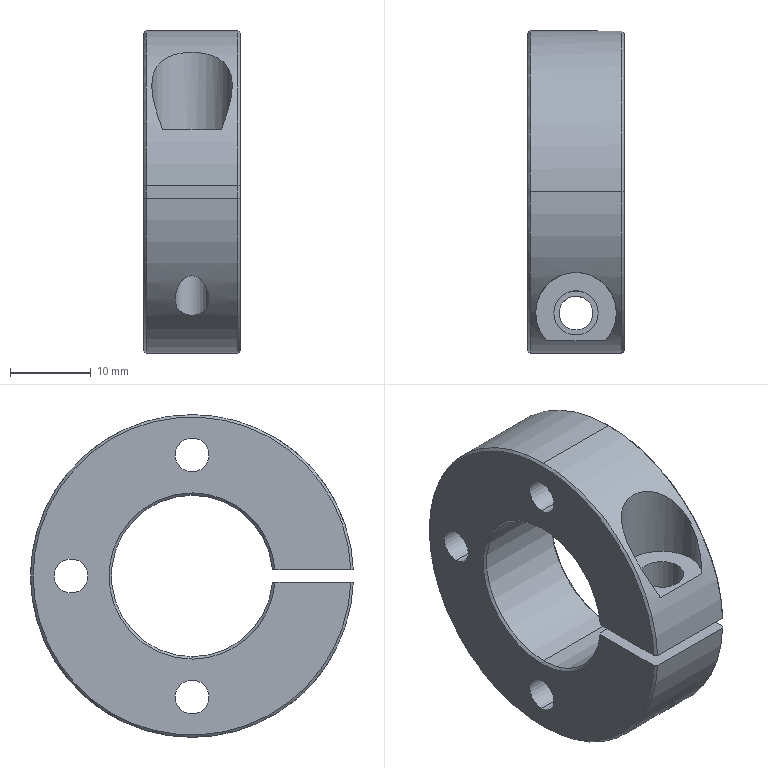Part | STEP file | SCSTR20-12_SCSTR20-12_1-2 | 1 solid | 35 faces | box 12 x 39.986 x 40 mm | volume 9883 mm3 | cylinder 19 | cone 11 | plane 5 | commonest cylinder face diameters 4.2 x8 10 x3 20 x3 40 x3 5.5 x2
STEP:
#1=CARTESIAN_POINT('',(-6.,0.,-17.1));
#2=VERTEX_POINT('',#1);
#3=CARTESIAN_POINT('',(-6.,0.,-12.9));
#4=VERTEX_POINT('',#3);
#5=CARTESIAN_POINT('',(-6.,0.,-15.));
#6=DIRECTION('',(-1.,0.,0.));
#7=DIRECTION('',(0.,0.,-1.));
#8=AXIS2_PLACEMENT_3D('',#5,#6,#7);
#9=CIRCLE('',#8,2.1);
#10=EDGE_CURVE('',#2,#4,#9,.T.);
#11=ORIENTED_EDGE('',*,*,#10,.T.);
#12=CARTESIAN_POINT('',(6.,0.,-12.9));
#13=VERTEX_POINT('',#12);
#14=CARTESIAN_POINT('',(6.,0.,-12.9));
#15=DIRECTION('',(1.,0.,0.));
#16=VECTOR('',#15,1000.);
#17=LINE('',#14,#16);
#18=EDGE_CURVE('',#4,#13,#17,.T.);
#19=ORIENTED_EDGE('',*,*,#18,.T.);
#20=CARTESIAN_POINT('',(6.,0.,-17.1));
#21=VERTEX_POINT('',#20);
#22=CARTESIAN_POINT('',(6.,0.,-15.));
#23=DIRECTION('',(-1.,0.,0.));
#24=DIRECTION('',(0.,0.,-1.));
#25=AXIS2_PLACEMENT_3D('',#22,#23,#24);
#26=CIRCLE('',#25,2.1);
#27=EDGE_CURVE('',#21,#13,#26,.T.);
#28=ORIENTED_EDGE('',*,*,#27,.F.);
#29=CARTESIAN_POINT('',(6.,0.,-17.1));
#30=DIRECTION('',(1.,0.,0.));
#31=VECTOR('',#30,1000.);
#32=LINE('',#29,#31);
#33=EDGE_CURVE('',#2,#21,#32,.T.);
#34=ORIENTED_EDGE('',*,*,#33,.F.);
#35=EDGE_LOOP('',(#11,#19,#28,#34));
#36=FACE_OUTER_BOUND('',#35,.T.);
#37=CARTESIAN_POINT('',(6.,0.,-15.));
#38=DIRECTION('',(1.,0.,0.));
#39=DIRECTION('',(0.,0.,-1.));
#40=AXIS2_PLACEMENT_3D('',#37,#38,#39);
#41=CYLINDRICAL_SURFACE('',#40,2.1);
#42=ADVANCED_FACE('',(#36),#41,.F.);
#43=CARTESIAN_POINT('',(-6.,0.,12.9));
#44=VERTEX_POINT('',#43);
#45=CARTESIAN_POINT('',(-6.,0.,17.1));
#46=VERTEX_POINT('',#45);
#47=CARTESIAN_POINT('',(-6.,0.,15.));
#48=DIRECTION('',(-1.,0.,0.));
#49=DIRECTION('',(0.,0.,-1.));
#50=AXIS2_PLACEMENT_3D('',#47,#48,#49);
#51=CIRCLE('',#50,2.1);
#52=EDGE_CURVE('',#44,#46,#51,.T.);
#53=ORIENTED_EDGE('',*,*,#52,.T.);
#54=CARTESIAN_POINT('',(6.,0.,17.1));
#55=VERTEX_POINT('',#54);
#56=CARTESIAN_POINT('',(6.,0.,17.1));
#57=DIRECTION('',(1.,0.,0.));
#58=VECTOR('',#57,1000.);
#59=LINE('',#56,#58);
#60=EDGE_CURVE('',#46,#55,#59,.T.);
#61=ORIENTED_EDGE('',*,*,#60,.T.);
#62=CARTESIAN_POINT('',(6.,0.,12.9));
#63=VERTEX_POINT('',#62);
#64=CARTESIAN_POINT('',(6.,0.,15.));
#65=DIRECTION('',(-1.,0.,0.));
#66=DIRECTION('',(0.,0.,-1.));
#67=AXIS2_PLACEMENT_3D('',#64,#65,#66);
#68=CIRCLE('',#67,2.1);
#69=EDGE_CURVE('',#63,#55,#68,.T.);
#70=ORIENTED_EDGE('',*,*,#69,.F.);
#71=CARTESIAN_POINT('',(6.,0.,12.9));
#72=DIRECTION('',(1.,0.,0.));
#73=VECTOR('',#72,1000.);
#74=LINE('',#71,#73);
#75=EDGE_CURVE('',#44,#63,#74,.T.);
#76=ORIENTED_EDGE('',*,*,#75,.F.);
#77=EDGE_LOOP('',(#53,#61,#70,#76));
#78=FACE_OUTER_BOUND('',#77,.T.);
#79=CARTESIAN_POINT('',(6.,0.,15.));
#80=DIRECTION('',(1.,0.,0.));
#81=DIRECTION('',(0.,0.,-1.));
#82=AXIS2_PLACEMENT_3D('',#79,#80,#81);
#83=CYLINDRICAL_SURFACE('',#82,2.1);
#84=ADVANCED_FACE('',(#78),#83,.F.);
#85=CARTESIAN_POINT('',(-6.,15.,-2.1));
#86=VERTEX_POINT('',#85);
#87=CARTESIAN_POINT('',(-6.,15.,2.1));
#88=VERTEX_POINT('',#87);
#89=CARTESIAN_POINT('',(-6.,15.,0.));
#90=DIRECTION('',(-1.,0.,0.));
#91=DIRECTION('',(0.,0.,-1.));
#92=AXIS2_PLACEMENT_3D('',#89,#90,#91);
#93=CIRCLE('',#92,2.1);
#94=EDGE_CURVE('',#86,#88,#93,.T.);
#95=ORIENTED_EDGE('',*,*,#94,.T.);
#96=CARTESIAN_POINT('',(6.,15.,2.1));
#97=VERTEX_POINT('',#96);
#98=CARTESIAN_POINT('',(6.,15.,2.1));
#99=DIRECTION('',(1.,0.,0.));
#100=VECTOR('',#99,1000.);
#101=LINE('',#98,#100);
#102=EDGE_CURVE('',#88,#97,#101,.T.);
#103=ORIENTED_EDGE('',*,*,#102,.T.);
#104=CARTESIAN_POINT('',(6.,15.,-2.1));
#105=VERTEX_POINT('',#104);
#106=CARTESIAN_POINT('',(6.,15.,0.));
#107=DIRECTION('',(-1.,0.,0.));
#108=DIRECTION('',(0.,0.,-1.));
#109=AXIS2_PLACEMENT_3D('',#106,#107,#108);
#110=CIRCLE('',#109,2.1);
#111=EDGE_CURVE('',#105,#97,#110,.T.);
#112=ORIENTED_EDGE('',*,*,#111,.F.);
#113=CARTESIAN_POINT('',(6.,15.,-2.1));
#114=DIRECTION('',(1.,0.,0.));
#115=VECTOR('',#114,1000.);
#116=LINE('',#113,#115);
#117=EDGE_CURVE('',#86,#105,#116,.T.);
#118=ORIENTED_EDGE('',*,*,#117,.F.);
#119=EDGE_LOOP('',(#95,#103,#112,#118));
#120=FACE_OUTER_BOUND('',#119,.T.);
#121=CARTESIAN_POINT('',(6.,15.,0.));
#122=DIRECTION('',(1.,0.,0.));
#123=DIRECTION('',(0.,0.,-1.));
#124=AXIS2_PLACEMENT_3D('',#121,#122,#123);
#125=CYLINDRICAL_SURFACE('',#124,2.1);
#126=ADVANCED_FACE('',(#120),#125,.F.);
#127=CARTESIAN_POINT('',(-5.7,0.,-10.));
#128=VERTEX_POINT('',#127);
#129=CARTESIAN_POINT('',(-5.7,-9.972,-0.75));
#130=VERTEX_POINT('',#129);
#131=CARTESIAN_POINT('',(-5.7,0.,0.));
#132=DIRECTION('',(-1.,0.,0.));
#133=DIRECTION('',(0.,0.,1.));
#134=AXIS2_PLACEMENT_3D('',#131,#132,#133);
#135=CIRCLE('',#134,10.);
#136=EDGE_CURVE('',#128,#130,#135,.T.);
#137=ORIENTED_EDGE('',*,*,#136,.F.);
#138=CARTESIAN_POINT('',(-6.,0.,-10.3));
#139=VERTEX_POINT('',#138);
#140=CARTESIAN_POINT('',(-6.,0.,-10.3));
#141=DIRECTION('',(-0.7071,0.,-0.7071));
#142=VECTOR('',#141,1000.);
#143=LINE('',#140,#142);
#144=EDGE_CURVE('',#128,#139,#143,.T.);
#145=ORIENTED_EDGE('',*,*,#144,.T.);
#146=CARTESIAN_POINT('',(-6.,-10.273,-0.75));
#147=VERTEX_POINT('',#146);
#148=CARTESIAN_POINT('',(-6.,0.,0.));
#149=DIRECTION('',(-1.,0.,0.));
#150=DIRECTION('',(0.,0.,1.));
#151=AXIS2_PLACEMENT_3D('',#148,#149,#150);
#152=CIRCLE('',#151,10.3);
#153=EDGE_CURVE('',#139,#147,#152,.T.);
#154=ORIENTED_EDGE('',*,*,#153,.T.);
#155=CARTESIAN_POINT('',(-6.,-10.273,-0.75));
#156=CARTESIAN_POINT('',(-5.9,-10.172,-0.75));
#157=CARTESIAN_POINT('',(-5.8,-10.072,-0.75));
#158=CARTESIAN_POINT('',(-5.7,-9.972,-0.75));
#159=B_SPLINE_CURVE_WITH_KNOTS('',3,(#155,#156,#157,#158),.UNSPECIFIED.,.F.,.F.,(4,4),(0.,0.0004248),.UNSPECIFIED.);
#160=EDGE_CURVE('',#147,#130,#159,.T.);
#161=ORIENTED_EDGE('',*,*,#160,.T.);
#162=EDGE_LOOP('',(#137,#145,#154,#161));
#163=FACE_OUTER_BOUND('',#162,.T.);
#164=CARTESIAN_POINT('',(-6.,0.,0.));
#165=DIRECTION('',(-1.,0.,0.));
#166=DIRECTION('',(0.,0.,1.));
#167=AXIS2_PLACEMENT_3D('',#164,#165,#166);
#168=CONICAL_SURFACE('',#167,10.3,0.7854);
#169=ADVANCED_FACE('',(#163),#168,.F.);
#170=ORIENTED_EDGE('',*,*,#144,.F.);
#171=CARTESIAN_POINT('',(-5.7,0.,10.));
#172=VERTEX_POINT('',#171);
#173=CARTESIAN_POINT('',(-5.7,0.,0.));
#174=DIRECTION('',(-1.,0.,0.));
#175=DIRECTION('',(0.,0.,1.));
#176=AXIS2_PLACEMENT_3D('',#173,#174,#175);
#177=CIRCLE('',#176,10.);
#178=EDGE_CURVE('',#172,#128,#177,.T.);
#179=ORIENTED_EDGE('',*,*,#178,.F.);
#180=CARTESIAN_POINT('',(-6.,0.,10.3));
#181=VERTEX_POINT('',#180);
#182=CARTESIAN_POINT('',(-6.,0.,10.3));
#183=DIRECTION('',(-0.7071,0.,0.7071));
#184=VECTOR('',#183,1000.);
#185=LINE('',#182,#184);
#186=EDGE_CURVE('',#172,#181,#185,.T.);
#187=ORIENTED_EDGE('',*,*,#186,.T.);
#188=CARTESIAN_POINT('',(-6.,0.,0.));
#189=DIRECTION('',(-1.,0.,0.));
#190=DIRECTION('',(0.,0.,1.));
#191=AXIS2_PLACEMENT_3D('',#188,#189,#190);
#192=CIRCLE('',#191,10.3);
#193=EDGE_CURVE('',#181,#139,#192,.T.);
#194=ORIENTED_EDGE('',*,*,#193,.T.);
#195=EDGE_LOOP('',(#170,#179,#187,#194));
#196=FACE_OUTER_BOUND('',#195,.T.);
#197=CARTESIAN_POINT('',(-6.,0.,0.));
#198=DIRECTION('',(-1.,0.,0.));
#199=DIRECTION('',(0.,0.,1.));
#200=AXIS2_PLACEMENT_3D('',#197,#198,#199);
#201=CONICAL_SURFACE('',#200,10.3,0.7854);
#202=ADVANCED_FACE('',(#196),#201,.F.);
#203=CARTESIAN_POINT('',(-6.,-19.686,-0.75));
#204=VERTEX_POINT('',#203);
#205=CARTESIAN_POINT('',(-6.,19.7,0.));
#206=VERTEX_POINT('',#205);
#207=CARTESIAN_POINT('',(-6.,0.,0.));
#208=DIRECTION('',(1.,0.,0.));
#209=DIRECTION('',(0.,0.,-1.));
#210=AXIS2_PLACEMENT_3D('',#207,#208,#209);
#211=CIRCLE('',#210,19.7);
#212=EDGE_CURVE('',#204,#206,#211,.T.);
#213=ORIENTED_EDGE('',*,*,#212,.T.);
#214=CARTESIAN_POINT('',(-5.7,20.,0.));
#215=VERTEX_POINT('',#214);
#216=CARTESIAN_POINT('',(-5.7,20.,0.));
#217=DIRECTION('',(0.7071,0.7071,0.));
#218=VECTOR('',#217,1000.);
#219=LINE('',#216,#218);
#220=EDGE_CURVE('',#206,#215,#219,.T.);
#221=ORIENTED_EDGE('',*,*,#220,.T.);
#222=CARTESIAN_POINT('',(-5.7,0.,-20.));
#223=VERTEX_POINT('',#222);
#224=CARTESIAN_POINT('',(-5.7,0.,0.));
#225=DIRECTION('',(-1.,0.,0.));
#226=DIRECTION('',(0.,0.,-1.));
#227=AXIS2_PLACEMENT_3D('',#224,#225,#226);
#228=CIRCLE('',#227,20.);
#229=EDGE_CURVE('',#215,#223,#228,.T.);
#230=ORIENTED_EDGE('',*,*,#229,.T.);
#231=CARTESIAN_POINT('',(-5.7,-19.986,-0.75));
#232=VERTEX_POINT('',#231);
#233=CARTESIAN_POINT('',(-5.7,0.,0.));
#234=DIRECTION('',(-1.,0.,0.));
#235=DIRECTION('',(0.,0.,-1.));
#236=AXIS2_PLACEMENT_3D('',#233,#234,#235);
#237=CIRCLE('',#236,20.);
#238=EDGE_CURVE('',#223,#232,#237,.T.);
#239=ORIENTED_EDGE('',*,*,#238,.T.);
#240=CARTESIAN_POINT('',(-5.7,-19.986,-0.75));
#241=CARTESIAN_POINT('',(-5.8,-19.886,-0.75));
#242=CARTESIAN_POINT('',(-5.9,-19.786,-0.75));
#243=CARTESIAN_POINT('',(-6.,-19.686,-0.75));
#244=B_SPLINE_CURVE_WITH_KNOTS('',3,(#240,#241,#242,#243),.UNSPECIFIED.,.F.,.F.,(4,4),(0.,0.0004244),.UNSPECIFIED.);
#245=EDGE_CURVE('',#232,#204,#244,.T.);
#246=ORIENTED_EDGE('',*,*,#245,.T.);
#247=EDGE_LOOP('',(#213,#221,#230,#239,#246));
#248=FACE_OUTER_BOUND('',#247,.T.);
#249=CARTESIAN_POINT('',(-5.7,0.,0.));
#250=DIRECTION('',(1.,0.,0.));
#251=DIRECTION('',(0.,1.,0.));
#252=AXIS2_PLACEMENT_3D('',#249,#250,#251);
#253=CONICAL_SURFACE('',#252,20.,0.7854);
#254=ADVANCED_FACE('',(#248),#253,.T.);
#255=CARTESIAN_POINT('',(-5.7,-9.972,0.75));
#256=VERTEX_POINT('',#255);
#257=CARTESIAN_POINT('',(-5.7,0.,0.));
#258=DIRECTION('',(-1.,0.,0.));
#259=DIRECTION('',(0.,0.,1.));
#260=AXIS2_PLACEMENT_3D('',#257,#258,#259);
#261=CIRCLE('',#260,10.);
#262=EDGE_CURVE('',#256,#172,#261,.T.);
#263=ORIENTED_EDGE('',*,*,#262,.T.);
#264=CARTESIAN_POINT('',(5.7,0.,10.));
#265=VERTEX_POINT('',#264);
#266=CARTESIAN_POINT('',(-6.,0.,10.));
#267=DIRECTION('',(1.,0.,0.));
#268=VECTOR('',#267,1000.);
#269=LINE('',#266,#268);
#270=EDGE_CURVE('',#172,#265,#269,.T.);
#271=ORIENTED_EDGE('',*,*,#270,.T.);
#272=CARTESIAN_POINT('',(5.7,-9.972,0.75));
#273=VERTEX_POINT('',#272);
#274=CARTESIAN_POINT('',(5.7,0.,0.));
#275=DIRECTION('',(-1.,0.,0.));
#276=DIRECTION('',(0.,0.,-1.));
#277=AXIS2_PLACEMENT_3D('',#274,#275,#276);
#278=CIRCLE('',#277,10.);
#279=EDGE_CURVE('',#273,#265,#278,.T.);
#280=ORIENTED_EDGE('',*,*,#279,.F.);
#281=CARTESIAN_POINT('',(-6.,-9.972,0.75));
#282=DIRECTION('',(-1.,0.,0.));
#283=VECTOR('',#282,1000.);
#284=LINE('',#281,#283);
#285=EDGE_CURVE('',#273,#256,#284,.T.);
#286=ORIENTED_EDGE('',*,*,#285,.T.);
#287=EDGE_LOOP('',(#263,#271,#280,#286));
#288=FACE_OUTER_BOUND('',#287,.T.);
#289=CARTESIAN_POINT('',(-6.,0.,0.));
#290=DIRECTION('',(1.,0.,0.));
#291=DIRECTION('',(0.,0.,-1.));
#292=AXIS2_PLACEMENT_3D('',#289,#290,#291);
#293=CYLINDRICAL_SURFACE('',#292,10.);
#294=ADVANCED_FACE('',(#288),#293,.F.);
#295=ORIENTED_EDGE('',*,*,#270,.F.);
#296=ORIENTED_EDGE('',*,*,#178,.T.);
#297=CARTESIAN_POINT('',(5.7,0.,-10.));
#298=VERTEX_POINT('',#297);
#299=CARTESIAN_POINT('',(-6.,0.,-10.));
#300=DIRECTION('',(1.,0.,0.));
#301=VECTOR('',#300,1000.);
#302=LINE('',#299,#301);
#303=EDGE_CURVE('',#128,#298,#302,.T.);
#304=ORIENTED_EDGE('',*,*,#303,.T.);
#305=CARTESIAN_POINT('',(5.7,0.,0.));
#306=DIRECTION('',(-1.,0.,0.));
#307=DIRECTION('',(0.,0.,-1.));
#308=AXIS2_PLACEMENT_3D('',#305,#306,#307);
#309=CIRCLE('',#308,10.);
#310=EDGE_CURVE('',#265,#298,#309,.T.);
#311=ORIENTED_EDGE('',*,*,#310,.F.);
#312=EDGE_LOOP('',(#295,#296,#304,#311));
#313=FACE_OUTER_BOUND('',#312,.T.);
#314=CARTESIAN_POINT('',(-6.,0.,0.));
#315=DIRECTION('',(1.,0.,0.));
#316=DIRECTION('',(0.,0.,-1.));
#317=AXIS2_PLACEMENT_3D('',#314,#315,#316);
#318=CYLINDRICAL_SURFACE('',#317,10.);
#319=ADVANCED_FACE('',(#313),#318,.F.);
#320=CARTESIAN_POINT('',(2.75,-15.,7.75));
#321=VERTEX_POINT('',#320);
#322=CARTESIAN_POINT('',(-2.75,-15.,7.75));
#323=VERTEX_POINT('',#322);
#324=CARTESIAN_POINT('',(0.,-15.,7.75));
#325=DIRECTION('',(0.,0.,-1.));
#326=DIRECTION('',(-1.,0.,0.));
#327=AXIS2_PLACEMENT_3D('',#324,#325,#326);
#328=CIRCLE('',#327,2.75);
#329=EDGE_CURVE('',#321,#323,#328,.T.);
#330=ORIENTED_EDGE('',*,*,#329,.F.);
#331=CARTESIAN_POINT('',(2.75,-15.,0.75));
#332=VERTEX_POINT('',#331);
#333=CARTESIAN_POINT('',(2.75,-15.,0.75));
#334=DIRECTION('',(0.,0.,-1.));
#335=VECTOR('',#334,1000.);
#336=LINE('',#333,#335);
#337=EDGE_CURVE('',#321,#332,#336,.T.);
#338=ORIENTED_EDGE('',*,*,#337,.T.);
#339=CARTESIAN_POINT('',(-2.75,-15.,0.75));
#340=VERTEX_POINT('',#339);
#341=CARTESIAN_POINT('',(0.,-15.,0.75));
#342=DIRECTION('',(0.,0.,-1.));
#343=DIRECTION('',(-1.,0.,0.));
#344=AXIS2_PLACEMENT_3D('',#341,#342,#343);
#345=CIRCLE('',#344,2.75);
#346=EDGE_CURVE('',#332,#340,#345,.T.);
#347=ORIENTED_EDGE('',*,*,#346,.T.);
#348=CARTESIAN_POINT('',(-2.75,-15.,0.75));
#349=DIRECTION('',(0.,0.,-1.));
#350=VECTOR('',#349,1000.);
#351=LINE('',#348,#350);
#352=EDGE_CURVE('',#323,#340,#351,.T.);
#353=ORIENTED_EDGE('',*,*,#352,.F.);
#354=EDGE_LOOP('',(#330,#338,#347,#353));
#355=FACE_OUTER_BOUND('',#354,.T.);
#356=CARTESIAN_POINT('',(0.,-15.,0.75));
#357=DIRECTION('',(0.,0.,-1.));
#358=DIRECTION('',(-1.,0.,0.));
#359=AXIS2_PLACEMENT_3D('',#356,#357,#358);
#360=CYLINDRICAL_SURFACE('',#359,2.75);
#361=ADVANCED_FACE('',(#355),#360,.F.);
#362=CARTESIAN_POINT('',(5.7,0.,20.));
#363=VERTEX_POINT('',#362);
#364=CARTESIAN_POINT('',(5.7,0.,-20.));
#365=VERTEX_POINT('',#364);
#366=CARTESIAN_POINT('',(5.7,0.,0.));
#367=DIRECTION('',(-1.,0.,0.));
#368=DIRECTION('',(0.,0.,1.));
#369=AXIS2_PLACEMENT_3D('',#366,#367,#368);
#370=CIRCLE('',#369,20.);
#371=EDGE_CURVE('',#363,#365,#370,.T.);
#372=ORIENTED_EDGE('',*,*,#371,.T.);
#373=CARTESIAN_POINT('',(6.,0.,-20.));
#374=DIRECTION('',(-1.,0.,0.));
#375=VECTOR('',#374,1000.);
#376=LINE('',#373,#375);
#377=EDGE_CURVE('',#365,#223,#376,.T.);
#378=ORIENTED_EDGE('',*,*,#377,.T.);
#379=ORIENTED_EDGE('',*,*,#229,.F.);
#380=CARTESIAN_POINT('',(-5.7,0.,20.));
#381=VERTEX_POINT('',#380);
#382=CARTESIAN_POINT('',(-5.7,0.,0.));
#383=DIRECTION('',(-1.,0.,0.));
#384=DIRECTION('',(0.,0.,-1.));
#385=AXIS2_PLACEMENT_3D('',#382,#383,#384);
#386=CIRCLE('',#385,20.);
#387=EDGE_CURVE('',#381,#215,#386,.T.);
#388=ORIENTED_EDGE('',*,*,#387,.F.);
#389=CARTESIAN_POINT('',(6.,0.,20.));
#390=DIRECTION('',(-1.,0.,0.));
#391=VECTOR('',#390,1000.);
#392=LINE('',#389,#391);
#393=EDGE_CURVE('',#363,#381,#392,.T.);
#394=ORIENTED_EDGE('',*,*,#393,.F.);
#395=EDGE_LOOP('',(#372,#378,#379,#388,#394));
#396=FACE_OUTER_BOUND('',#395,.T.);
#397=CARTESIAN_POINT('',(6.,0.,0.));
#398=DIRECTION('',(-1.,0.,0.));
#399=DIRECTION('',(0.,0.,1.));
#400=AXIS2_PLACEMENT_3D('',#397,#398,#399);
#401=CYLINDRICAL_SURFACE('',#400,20.);
#402=ADVANCED_FACE('',(#396),#401,.T.);
#403=CARTESIAN_POINT('',(-3.631,-18.437,7.75));
#404=VERTEX_POINT('',#403);
#405=CARTESIAN_POINT('',(-5.,-15.,13.229));
#406=VERTEX_POINT('',#405);
#407=CARTESIAN_POINT('',(-3.631,-18.437,7.75));
#408=CARTESIAN_POINT('',(-4.016,-18.03,8.718));
#409=CARTESIAN_POINT('',(-4.348,-17.547,9.658));
#410=CARTESIAN_POINT('',(-4.716,-16.691,11.033));
#411=CARTESIAN_POINT('',(-4.817,-16.383,11.485));
#412=CARTESIAN_POINT('',(-4.96,-15.719,12.378));
#413=CARTESIAN_POINT('',(-5.,-15.368,12.811));
#414=CARTESIAN_POINT('',(-5.,-15.,13.229));
#415=B_SPLINE_CURVE_WITH_KNOTS('',3,(#407,#408,#409,#410,#411,#412,#413,#414),.UNSPECIFIED.,.F.,.F.,(4,2,2,4),(-0.01582,-0.01247,-0.0108,-0.009124),.UNSPECIFIED.);
#416=EDGE_CURVE('',#404,#406,#415,.T.);
#417=ORIENTED_EDGE('',*,*,#416,.T.);
#418=CARTESIAN_POINT('',(5.,-15.,13.229));
#419=VERTEX_POINT('',#418);
#420=CARTESIAN_POINT('',(-5.,-15.,13.229));
#421=CARTESIAN_POINT('',(-5.,-14.75,13.513));
#422=CARTESIAN_POINT('',(-4.981,-14.491,13.79));
#423=CARTESIAN_POINT('',(-4.897,-13.957,14.33));
#424=CARTESIAN_POINT('',(-4.832,-13.684,14.59));
#425=CARTESIAN_POINT('',(-4.65,-13.139,15.083));
#426=CARTESIAN_POINT('',(-4.532,-12.865,15.317));
#427=CARTESIAN_POINT('',(-4.232,-12.319,15.76));
#428=CARTESIAN_POINT('',(-4.051,-12.05,15.965));
#429=CARTESIAN_POINT('',(-3.733,-11.669,16.243));
#430=CARTESIAN_POINT('',(-3.619,-11.546,16.332));
#431=CARTESIAN_POINT('',(-3.374,-11.306,16.499));
#432=CARTESIAN_POINT('',(-3.241,-11.189,16.578));
#433=CARTESIAN_POINT('',(-2.827,-10.861,16.796));
#434=CARTESIAN_POINT('',(-2.525,-10.669,16.918));
#435=CARTESIAN_POINT('',(-2.031,-10.427,17.067));
#436=CARTESIAN_POINT('',(-1.858,-10.354,17.111));
#437=CARTESIAN_POINT('',(-1.504,-10.228,17.187));
#438=CARTESIAN_POINT('',(-1.324,-10.175,17.218));
#439=CARTESIAN_POINT('',(-0.9586,-10.089,17.269));
#440=CARTESIAN_POINT('',(-0.7727,-10.056,17.288));
#441=CARTESIAN_POINT('',(-0.3947,-10.012,17.314));
#442=CARTESIAN_POINT('',(-0.2017,-10.,17.32));
#443=CARTESIAN_POINT('',(0.3765,-9.999,17.321));
#444=CARTESIAN_POINT('',(0.7534,-10.043,17.296));
#445=CARTESIAN_POINT('',(1.306,-10.17,17.221));
#446=CARTESIAN_POINT('',(1.489,-10.223,17.19));
#447=CARTESIAN_POINT('',(1.843,-10.348,17.115));
#448=CARTESIAN_POINT('',(2.014,-10.42,17.071));
#449=CARTESIAN_POINT('',(2.51,-10.66,16.923));
#450=CARTESIAN_POINT('',(2.821,-10.857,16.799));
#451=CARTESIAN_POINT('',(3.374,-11.293,16.508));
#452=CARTESIAN_POINT('',(3.619,-11.534,16.342));
#453=CARTESIAN_POINT('',(4.05,-12.049,15.967));
#454=CARTESIAN_POINT('',(4.229,-12.315,15.763));
#455=CARTESIAN_POINT('',(4.53,-12.86,15.321));
#456=CARTESIAN_POINT('',(4.65,-13.139,15.083));
#457=CARTESIAN_POINT('',(4.833,-13.686,14.588));
#458=CARTESIAN_POINT('',(4.897,-13.956,14.331));
#459=CARTESIAN_POINT('',(4.981,-14.486,13.795));
#460=CARTESIAN_POINT('',(5.,-14.748,13.515));
#461=CARTESIAN_POINT('',(5.,-15.,13.229));
#462=B_SPLINE_CURVE_WITH_KNOTS('',3,(#420,#421,#422,#423,#424,#425,#426,#427,#428,#429,#430,#431,#432,#433,#434,#435,#436,#437,#438,#439,#440,#441,#442,#443,#444,#445,#446,#447,#448,#449,#450,#451,#452,#453,#454,#455,#456,#457,#458,#459,#460,#461),.UNSPECIFIED.,.F.,.F.,(4,2,2,2,2,2,2,2,2,2,2,2,2,2,2,2,2,2,2,2,4),(-0.009124,-0.007984,-0.006845,-0.005706,-0.004566,-0.003997,-0.003427,-0.002288,-0.001718,-0.001148,-0.0005785,-0.00000887,0.00113,0.0017,0.00227,0.003409,0.004549,0.005688,0.006827,0.007967,0.009106),.UNSPECIFIED.);
#463=EDGE_CURVE('',#406,#419,#462,.T.);
#464=ORIENTED_EDGE('',*,*,#463,.T.);
#465=CARTESIAN_POINT('',(3.631,-18.437,7.75));
#466=VERTEX_POINT('',#465);
#467=CARTESIAN_POINT('',(5.,-15.,13.229));
#468=CARTESIAN_POINT('',(5.,-15.369,12.81));
#469=CARTESIAN_POINT('',(4.96,-15.717,12.381));
#470=CARTESIAN_POINT('',(4.82,-16.372,11.5));
#471=CARTESIAN_POINT('',(4.72,-16.68,11.049));
#472=CARTESIAN_POINT('',(4.473,-17.256,10.125));
#473=CARTESIAN_POINT('',(4.327,-17.522,9.657));
#474=CARTESIAN_POINT('',(4.003,-18.011,8.711));
#475=CARTESIAN_POINT('',(3.823,-18.234,8.234));
#476=CARTESIAN_POINT('',(3.631,-18.437,7.75));
#477=B_SPLINE_CURVE_WITH_KNOTS('',3,(#467,#468,#469,#470,#471,#472,#473,#474,#475,#476),.UNSPECIFIED.,.F.,.F.,(4,2,2,2,4),(0.009106,0.01078,0.01244,0.01411,0.01578),.UNSPECIFIED.);
#478=EDGE_CURVE('',#419,#466,#477,.T.);
#479=ORIENTED_EDGE('',*,*,#478,.T.);
#480=CARTESIAN_POINT('',(6.,-18.437,7.75));
#481=DIRECTION('',(-1.,0.,0.));
#482=VECTOR('',#481,1000.);
#483=LINE('',#480,#482);
#484=EDGE_CURVE('',#466,#404,#483,.T.);
#485=ORIENTED_EDGE('',*,*,#484,.T.);
#486=EDGE_LOOP('',(#417,#464,#479,#485));
#487=FACE_BOUND('',#486,.T.);
#488=CARTESIAN_POINT('',(5.7,-19.986,0.75));
#489=VERTEX_POINT('',#488);
#490=CARTESIAN_POINT('',(5.7,0.,0.));
#491=DIRECTION('',(-1.,0.,0.));
#492=DIRECTION('',(0.,0.,1.));
#493=AXIS2_PLACEMENT_3D('',#490,#491,#492);
#494=CIRCLE('',#493,20.);
#495=EDGE_CURVE('',#489,#363,#494,.T.);
#496=ORIENTED_EDGE('',*,*,#495,.T.);
#497=ORIENTED_EDGE('',*,*,#393,.T.);
#498=CARTESIAN_POINT('',(-5.7,-19.986,0.75));
#499=VERTEX_POINT('',#498);
#500=CARTESIAN_POINT('',(-5.7,0.,0.));
#501=DIRECTION('',(-1.,0.,0.));
#502=DIRECTION('',(0.,0.,-1.));
#503=AXIS2_PLACEMENT_3D('',#500,#501,#502);
#504=CIRCLE('',#503,20.);
#505=EDGE_CURVE('',#499,#381,#504,.T.);
#506=ORIENTED_EDGE('',*,*,#505,.F.);
#507=CARTESIAN_POINT('',(-6.,-19.986,0.75));
#508=DIRECTION('',(1.,0.,0.));
#509=VECTOR('',#508,1000.);
#510=LINE('',#507,#509);
#511=EDGE_CURVE('',#499,#489,#510,.T.);
#512=ORIENTED_EDGE('',*,*,#511,.T.);
#513=EDGE_LOOP('',(#496,#497,#506,#512));
#514=FACE_OUTER_BOUND('',#513,.T.);
#515=CARTESIAN_POINT('',(6.,0.,0.));
#516=DIRECTION('',(-1.,0.,0.));
#517=DIRECTION('',(0.,0.,1.));
#518=AXIS2_PLACEMENT_3D('',#515,#516,#517);
#519=CYLINDRICAL_SURFACE('',#518,20.);
#520=ADVANCED_FACE('',(#487,#514),#519,.T.);
#521=CARTESIAN_POINT('',(-2.1,-15.,-13.229));
#522=VERTEX_POINT('',#521);
#523=CARTESIAN_POINT('',(2.1,-15.,-13.229));
#524=VERTEX_POINT('',#523);
#525=CARTESIAN_POINT('',(-2.1,-15.,-13.229));
#526=CARTESIAN_POINT('',(-2.1,-15.248,-12.947));
#527=CARTESIAN_POINT('',(-2.057,-15.484,-12.664));
#528=CARTESIAN_POINT('',(-1.897,-15.932,-12.096));
#529=CARTESIAN_POINT('',(-1.777,-16.146,-11.807));
#530=CARTESIAN_POINT('',(-1.537,-16.436,-11.396));
#531=CARTESIAN_POINT('',(-1.447,-16.528,-11.262));
#532=CARTESIAN_POINT('',(-1.238,-16.702,-11.003));
#533=CARTESIAN_POINT('',(-1.121,-16.782,-10.88));
#534=CARTESIAN_POINT('',(-0.8546,-16.924,-10.658));
#535=CARTESIAN_POINT('',(-0.7046,-16.986,-10.559));
#536=CARTESIAN_POINT('',(-0.37,-17.074,-10.415));
#537=CARTESIAN_POINT('',(-0.183,-17.1,-10.372));
#538=CARTESIAN_POINT('',(0.1932,-17.1,-10.373));
#539=CARTESIAN_POINT('',(0.379,-17.073,-10.418));
#540=CARTESIAN_POINT('',(0.7112,-16.983,-10.563));
#541=CARTESIAN_POINT('',(0.8616,-16.921,-10.663));
#542=CARTESIAN_POINT('',(1.125,-16.779,-10.884));
#543=CARTESIAN_POINT('',(1.243,-16.698,-11.009));
#544=CARTESIAN_POINT('',(1.45,-16.525,-11.267));
#545=CARTESIAN_POINT('',(1.54,-16.434,-11.4));
#546=CARTESIAN_POINT('',(1.779,-16.144,-11.811));
#547=CARTESIAN_POINT('',(1.898,-15.93,-12.098));
#548=CARTESIAN_POINT('',(2.057,-15.483,-12.665));
#549=CARTESIAN_POINT('',(2.1,-15.248,-12.948));
#550=CARTESIAN_POINT('',(2.1,-15.,-13.229));
#551=B_SPLINE_CURVE_WITH_KNOTS('',3,(#525,#526,#527,#528,#529,#530,#531,#532,#533,#534,#535,#536,#537,#538,#539,#540,#541,#542,#543,#544,#545,#546,#547,#548,#549,#550),.UNSPECIFIED.,.F.,.F.,(4,2,2,2,2,2,2,2,2,2,2,2,4),(0.007926,0.009035,0.01014,0.0107,0.01125,0.01181,0.01236,0.01292,0.01347,0.01402,0.01458,0.01569,0.0168),.UNSPECIFIED.);
#552=EDGE_CURVE('',#522,#524,#551,.T.);
#553=ORIENTED_EDGE('',*,*,#552,.F.);
#554=CARTESIAN_POINT('',(-2.1,-15.,-0.75));
#555=VERTEX_POINT('',#554);
#556=CARTESIAN_POINT('',(-2.1,-15.,-0.75));
#557=DIRECTION('',(0.,0.,1.));
#558=VECTOR('',#557,1000.);
#559=LINE('',#556,#558);
#560=EDGE_CURVE('',#522,#555,#559,.T.);
#561=ORIENTED_EDGE('',*,*,#560,.T.);
#562=CARTESIAN_POINT('',(2.1,-15.,-0.75));
#563=VERTEX_POINT('',#562);
#564=CARTESIAN_POINT('',(0.,-15.,-0.75));
#565=DIRECTION('',(0.,0.,1.));
#566=DIRECTION('',(1.,0.,0.));
#567=AXIS2_PLACEMENT_3D('',#564,#565,#566);
#568=CIRCLE('',#567,2.1);
#569=EDGE_CURVE('',#555,#563,#568,.T.);
#570=ORIENTED_EDGE('',*,*,#569,.T.);
#571=CARTESIAN_POINT('',(2.1,-15.,-0.75));
#572=DIRECTION('',(0.,0.,1.));
#573=VECTOR('',#572,1000.);
#574=LINE('',#571,#573);
#575=EDGE_CURVE('',#524,#563,#574,.T.);
#576=ORIENTED_EDGE('',*,*,#575,.F.);
#577=EDGE_LOOP('',(#553,#561,#570,#576));
#578=FACE_OUTER_BOUND('',#577,.T.);
#579=CARTESIAN_POINT('',(0.,-15.,-0.75));
#580=DIRECTION('',(0.,0.,1.));
#581=DIRECTION('',(1.,0.,0.));
#582=AXIS2_PLACEMENT_3D('',#579,#580,#581);
#583=CYLINDRICAL_SURFACE('',#582,2.1);
#584=ADVANCED_FACE('',(#578),#583,.F.);
#585=CARTESIAN_POINT('',(6.,0.,-19.7));
#586=VERTEX_POINT('',#585);
#587=CARTESIAN_POINT('',(6.,0.,19.7));
#588=VERTEX_POINT('',#587);
#589=CARTESIAN_POINT('',(6.,0.,0.));
#590=DIRECTION('',(1.,0.,0.));
#591=DIRECTION('',(0.,0.,1.));
#592=AXIS2_PLACEMENT_3D('',#589,#590,#591);
#593=CIRCLE('',#592,19.7);
#594=EDGE_CURVE('',#586,#588,#593,.T.);
#595=ORIENTED_EDGE('',*,*,#594,.F.);
#596=CARTESIAN_POINT('',(5.7,0.,-20.));
#597=DIRECTION('',(-0.7071,0.,-0.7071));
#598=VECTOR('',#597,1000.);
#599=LINE('',#596,#598);
#600=EDGE_CURVE('',#586,#365,#599,.T.);
#601=ORIENTED_EDGE('',*,*,#600,.T.);
#602=ORIENTED_EDGE('',*,*,#371,.F.);
#603=CARTESIAN_POINT('',(5.7,0.,20.));
#604=DIRECTION('',(-0.7071,0.,0.7071));
#605=VECTOR('',#604,1000.);
#606=LINE('',#603,#605);
#607=EDGE_CURVE('',#588,#363,#606,.T.);
#608=ORIENTED_EDGE('',*,*,#607,.F.);
#609=EDGE_LOOP('',(#595,#601,#602,#608));
#610=FACE_OUTER_BOUND('',#609,.T.);
#611=CARTESIAN_POINT('',(5.7,0.,0.));
#612=DIRECTION('',(-1.,0.,0.));
#613=DIRECTION('',(0.,0.,1.));
#614=AXIS2_PLACEMENT_3D('',#611,#612,#613);
#615=CONICAL_SURFACE('',#614,20.,0.7854);
#616=ADVANCED_FACE('',(#610),#615,.T.);
#617=CARTESIAN_POINT('',(6.,-19.686,0.75));
#618=VERTEX_POINT('',#617);
#619=CARTESIAN_POINT('',(6.,0.,0.));
#620=DIRECTION('',(1.,0.,0.));
#621=DIRECTION('',(0.,0.,1.));
#622=AXIS2_PLACEMENT_3D('',#619,#620,#621);
#623=CIRCLE('',#622,19.7);
#624=EDGE_CURVE('',#588,#618,#623,.T.);
#625=ORIENTED_EDGE('',*,*,#624,.F.);
#626=ORIENTED_EDGE('',*,*,#607,.T.);
#627=ORIENTED_EDGE('',*,*,#495,.F.);
#628=CARTESIAN_POINT('',(5.7,-19.986,0.75));
#629=CARTESIAN_POINT('',(5.8,-19.886,0.75));
#630=CARTESIAN_POINT('',(5.9,-19.786,0.75));
#631=CARTESIAN_POINT('',(6.,-19.686,0.75));
#632=B_SPLINE_CURVE_WITH_KNOTS('',3,(#628,#629,#630,#631),.UNSPECIFIED.,.F.,.F.,(4,4),(0.,0.0004244),.UNSPECIFIED.);
#633=EDGE_CURVE('',#489,#618,#632,.T.);
#634=ORIENTED_EDGE('',*,*,#633,.T.);
#635=EDGE_LOOP('',(#625,#626,#627,#634));
#636=FACE_OUTER_BOUND('',#635,.T.);
#637=CARTESIAN_POINT('',(5.7,0.,0.));
#638=DIRECTION('',(-1.,0.,0.));
#639=DIRECTION('',(0.,0.,1.));
#640=AXIS2_PLACEMENT_3D('',#637,#638,#639);
#641=CONICAL_SURFACE('',#640,20.,0.7854);
#642=ADVANCED_FACE('',(#636),#641,.T.);
#643=ORIENTED_EDGE('',*,*,#279,.T.);
#644=CARTESIAN_POINT('',(6.,0.,10.3));
#645=VERTEX_POINT('',#644);
#646=CARTESIAN_POINT('',(6.,0.,10.3));
#647=DIRECTION('',(0.7071,0.,0.7071));
#648=VECTOR('',#647,1000.);
#649=LINE('',#646,#648);
#650=EDGE_CURVE('',#265,#645,#649,.T.);
#651=ORIENTED_EDGE('',*,*,#650,.T.);
#652=CARTESIAN_POINT('',(6.,-10.273,0.75));
#653=VERTEX_POINT('',#652);
#654=CARTESIAN_POINT('',(6.,0.,0.));
#655=DIRECTION('',(-1.,0.,0.));
#656=DIRECTION('',(0.,0.,-1.));
#657=AXIS2_PLACEMENT_3D('',#654,#655,#656);
#658=CIRCLE('',#657,10.3);
#659=EDGE_CURVE('',#653,#645,#658,.T.);
#660=ORIENTED_EDGE('',*,*,#659,.F.);
#661=CARTESIAN_POINT('',(5.7,-9.972,0.75));
#662=CARTESIAN_POINT('',(5.8,-10.072,0.75));
#663=CARTESIAN_POINT('',(5.9,-10.172,0.75));
#664=CARTESIAN_POINT('',(6.,-10.273,0.75));
#665=B_SPLINE_CURVE_WITH_KNOTS('',3,(#661,#662,#663,#664),.UNSPECIFIED.,.F.,.F.,(4,4),(0.,0.0004248),.UNSPECIFIED.);
#666=EDGE_CURVE('',#273,#653,#665,.T.);
#667=ORIENTED_EDGE('',*,*,#666,.F.);
#668=EDGE_LOOP('',(#643,#651,#660,#667));
#669=FACE_OUTER_BOUND('',#668,.T.);
#670=CARTESIAN_POINT('',(6.,0.,0.));
#671=DIRECTION('',(1.,0.,0.));
#672=DIRECTION('',(0.,0.,-1.));
#673=AXIS2_PLACEMENT_3D('',#670,#671,#672);
#674=CONICAL_SURFACE('',#673,10.3,0.7854);
#675=ADVANCED_FACE('',(#669),#674,.F.);
#676=ORIENTED_EDGE('',*,*,#650,.F.);
#677=ORIENTED_EDGE('',*,*,#310,.T.);
#678=CARTESIAN_POINT('',(6.,0.,-10.3));
#679=VERTEX_POINT('',#678);
#680=CARTESIAN_POINT('',(6.,0.,-10.3));
#681=DIRECTION('',(0.7071,0.,-0.7071));
#682=VECTOR('',#681,1000.);
#683=LINE('',#680,#682);
#684=EDGE_CURVE('',#298,#679,#683,.T.);
#685=ORIENTED_EDGE('',*,*,#684,.T.);
#686=CARTESIAN_POINT('',(6.,0.,0.));
#687=DIRECTION('',(-1.,0.,0.));
#688=DIRECTION('',(0.,0.,-1.));
#689=AXIS2_PLACEMENT_3D('',#686,#687,#688);
#690=CIRCLE('',#689,10.3);
#691=EDGE_CURVE('',#645,#679,#690,.T.);
#692=ORIENTED_EDGE('',*,*,#691,.F.);
#693=EDGE_LOOP('',(#676,#677,#685,#692));
#694=FACE_OUTER_BOUND('',#693,.T.);
#695=CARTESIAN_POINT('',(6.,0.,0.));
#696=DIRECTION('',(1.,0.,0.));
#697=DIRECTION('',(0.,0.,-1.));
#698=AXIS2_PLACEMENT_3D('',#695,#696,#697);
#699=CONICAL_SURFACE('',#698,10.3,0.7854);
#700=ADVANCED_FACE('',(#694),#699,.F.);
#701=ORIENTED_EDGE('',*,*,#478,.F.);
#702=CARTESIAN_POINT('',(5.,-15.,7.75));
#703=VERTEX_POINT('',#702);
#704=CARTESIAN_POINT('',(5.,-15.,22.75));
#705=DIRECTION('',(0.,0.,-1.));
#706=VECTOR('',#705,1000.);
#707=LINE('',#704,#706);
#708=EDGE_CURVE('',#419,#703,#707,.T.);
#709=ORIENTED_EDGE('',*,*,#708,.T.);
#710=CARTESIAN_POINT('',(0.,-15.,7.75));
#711=DIRECTION('',(0.,0.,-1.));
#712=DIRECTION('',(-1.,0.,0.));
#713=AXIS2_PLACEMENT_3D('',#710,#711,#712);
#714=CIRCLE('',#713,5.);
#715=EDGE_CURVE('',#703,#466,#714,.T.);
#716=ORIENTED_EDGE('',*,*,#715,.T.);
#717=EDGE_LOOP('',(#701,#709,#716));
#718=FACE_OUTER_BOUND('',#717,.T.);
#719=CARTESIAN_POINT('',(0.,-15.,22.75));
#720=DIRECTION('',(0.,0.,-1.));
#721=DIRECTION('',(-1.,0.,0.));
#722=AXIS2_PLACEMENT_3D('',#719,#720,#721);
#723=CYLINDRICAL_SURFACE('',#722,5.);
#724=ADVANCED_FACE('',(#718),#723,.F.);
#725=ORIENTED_EDGE('',*,*,#708,.F.);
#726=ORIENTED_EDGE('',*,*,#463,.F.);
#727=CARTESIAN_POINT('',(-5.,-15.,7.75));
#728=VERTEX_POINT('',#727);
#729=CARTESIAN_POINT('',(-5.,-15.,22.75));
#730=DIRECTION('',(0.,0.,-1.));
#731=VECTOR('',#730,1000.);
#732=LINE('',#729,#731);
#733=EDGE_CURVE('',#406,#728,#732,.T.);
#734=ORIENTED_EDGE('',*,*,#733,.T.);
#735=CARTESIAN_POINT('',(0.,-15.,7.75));
#736=DIRECTION('',(0.,0.,-1.));
#737=DIRECTION('',(-1.,0.,0.));
#738=AXIS2_PLACEMENT_3D('',#735,#736,#737);
#739=CIRCLE('',#738,5.);
#740=EDGE_CURVE('',#728,#703,#739,.T.);
#741=ORIENTED_EDGE('',*,*,#740,.T.);
#742=EDGE_LOOP('',(#725,#726,#734,#741));
#743=FACE_OUTER_BOUND('',#742,.T.);
#744=CARTESIAN_POINT('',(0.,-15.,22.75));
#745=DIRECTION('',(0.,0.,-1.));
#746=DIRECTION('',(-1.,0.,0.));
#747=AXIS2_PLACEMENT_3D('',#744,#745,#746);
#748=CYLINDRICAL_SURFACE('',#747,5.);
#749=ADVANCED_FACE('',(#743),#748,.F.);
#750=ORIENTED_EDGE('',*,*,#10,.F.);
#751=CARTESIAN_POINT('',(-6.,0.,-15.));
#752=DIRECTION('',(-1.,0.,0.));
#753=DIRECTION('',(0.,0.,-1.));
#754=AXIS2_PLACEMENT_3D('',#751,#752,#753);
#755=CIRCLE('',#754,2.1);
#756=EDGE_CURVE('',#4,#2,#755,.T.);
#757=ORIENTED_EDGE('',*,*,#756,.F.);
#758=EDGE_LOOP('',(#750,#757));
#759=FACE_BOUND('',#758,.T.);
#760=ORIENTED_EDGE('',*,*,#52,.F.);
#761=CARTESIAN_POINT('',(-6.,0.,15.));
#762=DIRECTION('',(-1.,0.,0.));
#763=DIRECTION('',(0.,0.,-1.));
#764=AXIS2_PLACEMENT_3D('',#761,#762,#763);
#765=CIRCLE('',#764,2.1);
#766=EDGE_CURVE('',#46,#44,#765,.T.);
#767=ORIENTED_EDGE('',*,*,#766,.F.);
#768=EDGE_LOOP('',(#760,#767));
#769=FACE_BOUND('',#768,.T.);
#770=ORIENTED_EDGE('',*,*,#94,.F.);
#771=CARTESIAN_POINT('',(-6.,15.,0.));
#772=DIRECTION('',(-1.,0.,0.));
#773=DIRECTION('',(0.,0.,-1.));
#774=AXIS2_PLACEMENT_3D('',#771,#772,#773);
#775=CIRCLE('',#774,2.1);
#776=EDGE_CURVE('',#88,#86,#775,.T.);
#777=ORIENTED_EDGE('',*,*,#776,.F.);
#778=EDGE_LOOP('',(#770,#777));
#779=FACE_BOUND('',#778,.T.);
#780=CARTESIAN_POINT('',(-6.,-10.273,0.75));
#781=VERTEX_POINT('',#780);
#782=CARTESIAN_POINT('',(-6.,0.,0.));
#783=DIRECTION('',(-1.,0.,0.));
#784=DIRECTION('',(0.,0.,1.));
#785=AXIS2_PLACEMENT_3D('',#782,#783,#784);
#786=CIRCLE('',#785,10.3);
#787=EDGE_CURVE('',#781,#181,#786,.T.);
#788=ORIENTED_EDGE('',*,*,#787,.F.);
#789=CARTESIAN_POINT('',(-6.,-19.686,0.75));
#790=VERTEX_POINT('',#789);
#791=CARTESIAN_POINT('',(-6.,0.,0.75));
#792=DIRECTION('',(0.,1.,0.));
#793=VECTOR('',#792,1000.);
#794=LINE('',#791,#793);
#795=EDGE_CURVE('',#790,#781,#794,.T.);
#796=ORIENTED_EDGE('',*,*,#795,.F.);
#797=CARTESIAN_POINT('',(-6.,0.,0.));
#798=DIRECTION('',(1.,0.,0.));
#799=DIRECTION('',(0.,0.,-1.));
#800=AXIS2_PLACEMENT_3D('',#797,#798,#799);
#801=CIRCLE('',#800,19.7);
#802=EDGE_CURVE('',#206,#790,#801,.T.);
#803=ORIENTED_EDGE('',*,*,#802,.F.);
#804=ORIENTED_EDGE('',*,*,#212,.F.);
#805=CARTESIAN_POINT('',(-6.,0.,-0.75));
#806=DIRECTION('',(0.,-1.,0.));
#807=VECTOR('',#806,1000.);
#808=LINE('',#805,#807);
#809=EDGE_CURVE('',#147,#204,#808,.T.);
#810=ORIENTED_EDGE('',*,*,#809,.F.);
#811=ORIENTED_EDGE('',*,*,#153,.F.);
#812=ORIENTED_EDGE('',*,*,#193,.F.);
#813=EDGE_LOOP('',(#788,#796,#803,#804,#810,#811,#812));
#814=FACE_OUTER_BOUND('',#813,.T.);
#815=CARTESIAN_POINT('',(-6.,0.,0.));
#816=DIRECTION('',(1.,0.,0.));
#817=DIRECTION('',(0.,0.,-1.));
#818=AXIS2_PLACEMENT_3D('',#815,#816,#817);
#819=PLANE('',#818);
#820=ADVANCED_FACE('',(#759,#769,#779,#814),#819,.F.);
#821=ORIENTED_EDGE('',*,*,#18,.F.);
#822=ORIENTED_EDGE('',*,*,#756,.T.);
#823=ORIENTED_EDGE('',*,*,#33,.T.);
#824=CARTESIAN_POINT('',(6.,0.,-15.));
#825=DIRECTION('',(-1.,0.,0.));
#826=DIRECTION('',(0.,0.,-1.));
#827=AXIS2_PLACEMENT_3D('',#824,#825,#826);
#828=CIRCLE('',#827,2.1);
#829=EDGE_CURVE('',#13,#21,#828,.T.);
#830=ORIENTED_EDGE('',*,*,#829,.F.);
#831=EDGE_LOOP('',(#821,#822,#823,#830));
#832=FACE_OUTER_BOUND('',#831,.T.);
#833=CARTESIAN_POINT('',(6.,0.,-15.));
#834=DIRECTION('',(1.,0.,0.));
#835=DIRECTION('',(0.,0.,-1.));
#836=AXIS2_PLACEMENT_3D('',#833,#834,#835);
#837=CYLINDRICAL_SURFACE('',#836,2.1);
#838=ADVANCED_FACE('',(#832),#837,.F.);
#839=ORIENTED_EDGE('',*,*,#60,.F.);
#840=ORIENTED_EDGE('',*,*,#766,.T.);
#841=ORIENTED_EDGE('',*,*,#75,.T.);
#842=CARTESIAN_POINT('',(6.,0.,15.));
#843=DIRECTION('',(-1.,0.,0.));
#844=DIRECTION('',(0.,0.,-1.));
#845=AXIS2_PLACEMENT_3D('',#842,#843,#844);
#846=CIRCLE('',#845,2.1);
#847=EDGE_CURVE('',#55,#63,#846,.T.);
#848=ORIENTED_EDGE('',*,*,#847,.F.);
#849=EDGE_LOOP('',(#839,#840,#841,#848));
#850=FACE_OUTER_BOUND('',#849,.T.);
#851=CARTESIAN_POINT('',(6.,0.,15.));
#852=DIRECTION('',(1.,0.,0.));
#853=DIRECTION('',(0.,0.,-1.));
#854=AXIS2_PLACEMENT_3D('',#851,#852,#853);
#855=CYLINDRICAL_SURFACE('',#854,2.1);
#856=ADVANCED_FACE('',(#850),#855,.F.);
#857=ORIENTED_EDGE('',*,*,#102,.F.);
#858=ORIENTED_EDGE('',*,*,#776,.T.);
#859=ORIENTED_EDGE('',*,*,#117,.T.);
#860=CARTESIAN_POINT('',(6.,15.,0.));
#861=DIRECTION('',(-1.,0.,0.));
#862=DIRECTION('',(0.,0.,-1.));
#863=AXIS2_PLACEMENT_3D('',#860,#861,#862);
#864=CIRCLE('',#863,2.1);
#865=EDGE_CURVE('',#97,#105,#864,.T.);
#866=ORIENTED_EDGE('',*,*,#865,.F.);
#867=EDGE_LOOP('',(#857,#858,#859,#866));
#868=FACE_OUTER_BOUND('',#867,.T.);
#869=CARTESIAN_POINT('',(6.,15.,0.));
#870=DIRECTION('',(1.,0.,0.));
#871=DIRECTION('',(0.,0.,-1.));
#872=AXIS2_PLACEMENT_3D('',#869,#870,#871);
#873=CYLINDRICAL_SURFACE('',#872,2.1);
#874=ADVANCED_FACE('',(#868),#873,.F.);
#875=ORIENTED_EDGE('',*,*,#186,.F.);
#876=ORIENTED_EDGE('',*,*,#262,.F.);
#877=CARTESIAN_POINT('',(-6.,-10.273,0.75));
#878=CARTESIAN_POINT('',(-5.9,-10.172,0.75));
#879=CARTESIAN_POINT('',(-5.8,-10.072,0.75));
#880=CARTESIAN_POINT('',(-5.7,-9.972,0.75));
#881=B_SPLINE_CURVE_WITH_KNOTS('',3,(#877,#878,#879,#880),.UNSPECIFIED.,.F.,.F.,(4,4),(0.,0.0004248),.UNSPECIFIED.);
#882=EDGE_CURVE('',#781,#256,#881,.T.);
#883=ORIENTED_EDGE('',*,*,#882,.F.);
#884=ORIENTED_EDGE('',*,*,#787,.T.);
#885=EDGE_LOOP('',(#875,#876,#883,#884));
#886=FACE_OUTER_BOUND('',#885,.T.);
#887=CARTESIAN_POINT('',(-6.,0.,0.));
#888=DIRECTION('',(-1.,0.,0.));
#889=DIRECTION('',(0.,0.,1.));
#890=AXIS2_PLACEMENT_3D('',#887,#888,#889);
#891=CONICAL_SURFACE('',#890,10.3,0.7854);
#892=ADVANCED_FACE('',(#886),#891,.F.);
#893=CARTESIAN_POINT('',(0.,-15.,0.75));
#894=DIRECTION('',(0.,0.,-1.));
#895=DIRECTION('',(-1.,0.,0.));
#896=AXIS2_PLACEMENT_3D('',#893,#894,#895);
#897=CIRCLE('',#896,2.75);
#898=EDGE_CURVE('',#340,#332,#897,.T.);
#899=ORIENTED_EDGE('',*,*,#898,.F.);
#900=ORIENTED_EDGE('',*,*,#346,.F.);
#901=EDGE_LOOP('',(#899,#900));
#902=FACE_BOUND('',#901,.T.);
#903=ORIENTED_EDGE('',*,*,#633,.F.);
#904=ORIENTED_EDGE('',*,*,#511,.F.);
#905=CARTESIAN_POINT('',(-6.,-19.686,0.75));
#906=CARTESIAN_POINT('',(-5.9,-19.786,0.75));
#907=CARTESIAN_POINT('',(-5.8,-19.886,0.75));
#908=CARTESIAN_POINT('',(-5.7,-19.986,0.75));
#909=B_SPLINE_CURVE_WITH_KNOTS('',3,(#905,#906,#907,#908),.UNSPECIFIED.,.F.,.F.,(4,4),(0.,0.0004244),.UNSPECIFIED.);
#910=EDGE_CURVE('',#790,#499,#909,.T.);
#911=ORIENTED_EDGE('',*,*,#910,.F.);
#912=ORIENTED_EDGE('',*,*,#795,.T.);
#913=ORIENTED_EDGE('',*,*,#882,.T.);
#914=ORIENTED_EDGE('',*,*,#285,.F.);
#915=ORIENTED_EDGE('',*,*,#666,.T.);
#916=CARTESIAN_POINT('',(6.,-3.453,0.75));
#917=DIRECTION('',(0.,1.,0.));
#918=VECTOR('',#917,1000.);
#919=LINE('',#916,#918);
#920=EDGE_CURVE('',#618,#653,#919,.T.);
#921=ORIENTED_EDGE('',*,*,#920,.F.);
#922=EDGE_LOOP('',(#903,#904,#911,#912,#913,#914,#915,#921));
#923=FACE_OUTER_BOUND('',#922,.T.);
#924=CARTESIAN_POINT('',(-6.,-3.453,0.75));
#925=DIRECTION('',(0.,0.,1.));
#926=DIRECTION('',(1.,0.,0.));
#927=AXIS2_PLACEMENT_3D('',#924,#925,#926);
#928=PLANE('',#927);
#929=ADVANCED_FACE('',(#902,#923),#928,.F.);
#930=ORIENTED_EDGE('',*,*,#220,.F.);
#931=ORIENTED_EDGE('',*,*,#802,.T.);
#932=ORIENTED_EDGE('',*,*,#910,.T.);
#933=ORIENTED_EDGE('',*,*,#505,.T.);
#934=ORIENTED_EDGE('',*,*,#387,.T.);
#935=EDGE_LOOP('',(#930,#931,#932,#933,#934));
#936=FACE_OUTER_BOUND('',#935,.T.);
#937=CARTESIAN_POINT('',(-5.7,0.,0.));
#938=DIRECTION('',(1.,0.,0.));
#939=DIRECTION('',(0.,1.,0.));
#940=AXIS2_PLACEMENT_3D('',#937,#938,#939);
#941=CONICAL_SURFACE('',#940,20.,0.7854);
#942=ADVANCED_FACE('',(#936),#941,.T.);
#943=CARTESIAN_POINT('',(0.,-15.,-0.75));
#944=DIRECTION('',(0.,0.,1.));
#945=DIRECTION('',(1.,0.,0.));
#946=AXIS2_PLACEMENT_3D('',#943,#944,#945);
#947=CIRCLE('',#946,2.1);
#948=EDGE_CURVE('',#563,#555,#947,.T.);
#949=ORIENTED_EDGE('',*,*,#948,.F.);
#950=ORIENTED_EDGE('',*,*,#569,.F.);
#951=EDGE_LOOP('',(#949,#950));
#952=FACE_BOUND('',#951,.T.);
#953=ORIENTED_EDGE('',*,*,#160,.F.);
#954=ORIENTED_EDGE('',*,*,#809,.T.);
#955=ORIENTED_EDGE('',*,*,#245,.F.);
#956=CARTESIAN_POINT('',(5.7,-19.986,-0.75));
#957=VERTEX_POINT('',#956);
#958=CARTESIAN_POINT('',(-6.,-19.986,-0.75));
#959=DIRECTION('',(-1.,0.,0.));
#960=VECTOR('',#959,1000.);
#961=LINE('',#958,#960);
#962=EDGE_CURVE('',#957,#232,#961,.T.);
#963=ORIENTED_EDGE('',*,*,#962,.F.);
#964=CARTESIAN_POINT('',(6.,-19.686,-0.75));
#965=VERTEX_POINT('',#964);
#966=CARTESIAN_POINT('',(6.,-19.686,-0.75));
#967=CARTESIAN_POINT('',(5.9,-19.786,-0.75));
#968=CARTESIAN_POINT('',(5.8,-19.886,-0.75));
#969=CARTESIAN_POINT('',(5.7,-19.986,-0.75));
#970=B_SPLINE_CURVE_WITH_KNOTS('',3,(#966,#967,#968,#969),.UNSPECIFIED.,.F.,.F.,(4,4),(0.,0.0004244),.UNSPECIFIED.);
#971=EDGE_CURVE('',#965,#957,#970,.T.);
#972=ORIENTED_EDGE('',*,*,#971,.F.);
#973=CARTESIAN_POINT('',(6.,-10.273,-0.75));
#974=VERTEX_POINT('',#973);
#975=CARTESIAN_POINT('',(6.,-3.453,-0.75));
#976=DIRECTION('',(0.,-1.,0.));
#977=VECTOR('',#976,1000.);
#978=LINE('',#975,#977);
#979=EDGE_CURVE('',#974,#965,#978,.T.);
#980=ORIENTED_EDGE('',*,*,#979,.F.);
#981=CARTESIAN_POINT('',(5.7,-9.972,-0.75));
#982=VERTEX_POINT('',#981);
#983=CARTESIAN_POINT('',(6.,-10.273,-0.75));
#984=CARTESIAN_POINT('',(5.9,-10.172,-0.75));
#985=CARTESIAN_POINT('',(5.8,-10.072,-0.75));
#986=CARTESIAN_POINT('',(5.7,-9.972,-0.75));
#987=B_SPLINE_CURVE_WITH_KNOTS('',3,(#983,#984,#985,#986),.UNSPECIFIED.,.F.,.F.,(4,4),(0.,0.0004248),.UNSPECIFIED.);
#988=EDGE_CURVE('',#974,#982,#987,.T.);
#989=ORIENTED_EDGE('',*,*,#988,.T.);
#990=CARTESIAN_POINT('',(-6.,-9.972,-0.75));
#991=DIRECTION('',(1.,0.,0.));
#992=VECTOR('',#991,1000.);
#993=LINE('',#990,#992);
#994=EDGE_CURVE('',#130,#982,#993,.T.);
#995=ORIENTED_EDGE('',*,*,#994,.F.);
#996=EDGE_LOOP('',(#953,#954,#955,#963,#972,#980,#989,#995));
#997=FACE_OUTER_BOUND('',#996,.T.);
#998=CARTESIAN_POINT('',(-6.,-3.453,-0.75));
#999=DIRECTION('',(0.,0.,-1.));
#1000=DIRECTION('',(-1.,0.,0.));
#1001=AXIS2_PLACEMENT_3D('',#998,#999,#1000);
#1002=PLANE('',#1001);
#1003=ADVANCED_FACE('',(#952,#997),#1002,.F.);
#1004=ORIENTED_EDGE('',*,*,#27,.T.);
#1005=ORIENTED_EDGE('',*,*,#829,.T.);
#1006=EDGE_LOOP('',(#1004,#1005));
#1007=FACE_BOUND('',#1006,.T.);
#1008=ORIENTED_EDGE('',*,*,#69,.T.);
#1009=ORIENTED_EDGE('',*,*,#847,.T.);
#1010=EDGE_LOOP('',(#1008,#1009));
#1011=FACE_BOUND('',#1010,.T.);
#1012=ORIENTED_EDGE('',*,*,#111,.T.);
#1013=ORIENTED_EDGE('',*,*,#865,.T.);
#1014=EDGE_LOOP('',(#1012,#1013));
#1015=FACE_BOUND('',#1014,.T.);
#1016=CARTESIAN_POINT('',(6.,0.,0.));
#1017=DIRECTION('',(1.,0.,0.));
#1018=DIRECTION('',(0.,0.,1.));
#1019=AXIS2_PLACEMENT_3D('',#1016,#1017,#1018);
#1020=CIRCLE('',#1019,19.7);
#1021=EDGE_CURVE('',#965,#586,#1020,.T.);
#1022=ORIENTED_EDGE('',*,*,#1021,.T.);
#1023=ORIENTED_EDGE('',*,*,#594,.T.);
#1024=ORIENTED_EDGE('',*,*,#624,.T.);
#1025=ORIENTED_EDGE('',*,*,#920,.T.);
#1026=ORIENTED_EDGE('',*,*,#659,.T.);
#1027=ORIENTED_EDGE('',*,*,#691,.T.);
#1028=CARTESIAN_POINT('',(6.,0.,0.));
#1029=DIRECTION('',(-1.,0.,0.));
#1030=DIRECTION('',(0.,0.,-1.));
#1031=AXIS2_PLACEMENT_3D('',#1028,#1029,#1030);
#1032=CIRCLE('',#1031,10.3);
#1033=EDGE_CURVE('',#679,#974,#1032,.T.);
#1034=ORIENTED_EDGE('',*,*,#1033,.T.);
#1035=ORIENTED_EDGE('',*,*,#979,.T.);
#1036=EDGE_LOOP('',(#1022,#1023,#1024,#1025,#1026,#1027,#1034,#1035));
#1037=FACE_OUTER_BOUND('',#1036,.T.);
#1038=CARTESIAN_POINT('',(6.,0.,0.));
#1039=DIRECTION('',(1.,0.,0.));
#1040=DIRECTION('',(0.,0.,-1.));
#1041=AXIS2_PLACEMENT_3D('',#1038,#1039,#1040);
#1042=PLANE('',#1041);
#1043=ADVANCED_FACE('',(#1007,#1011,#1015,#1037),#1042,.T.);
#1044=ORIENTED_EDGE('',*,*,#303,.F.);
#1045=ORIENTED_EDGE('',*,*,#136,.T.);
#1046=ORIENTED_EDGE('',*,*,#994,.T.);
#1047=CARTESIAN_POINT('',(5.7,0.,0.));
#1048=DIRECTION('',(-1.,0.,0.));
#1049=DIRECTION('',(0.,0.,-1.));
#1050=AXIS2_PLACEMENT_3D('',#1047,#1048,#1049);
#1051=CIRCLE('',#1050,10.);
#1052=EDGE_CURVE('',#298,#982,#1051,.T.);
#1053=ORIENTED_EDGE('',*,*,#1052,.F.);
#1054=EDGE_LOOP('',(#1044,#1045,#1046,#1053));
#1055=FACE_OUTER_BOUND('',#1054,.T.);
#1056=CARTESIAN_POINT('',(-6.,0.,0.));
#1057=DIRECTION('',(1.,0.,0.));
#1058=DIRECTION('',(0.,0.,-1.));
#1059=AXIS2_PLACEMENT_3D('',#1056,#1057,#1058);
#1060=CYLINDRICAL_SURFACE('',#1059,10.);
#1061=ADVANCED_FACE('',(#1055),#1060,.F.);
#1062=ORIENTED_EDGE('',*,*,#337,.F.);
#1063=CARTESIAN_POINT('',(0.,-15.,7.75));
#1064=DIRECTION('',(0.,0.,-1.));
#1065=DIRECTION('',(-1.,0.,0.));
#1066=AXIS2_PLACEMENT_3D('',#1063,#1064,#1065);
#1067=CIRCLE('',#1066,2.75);
#1068=EDGE_CURVE('',#323,#321,#1067,.T.);
#1069=ORIENTED_EDGE('',*,*,#1068,.F.);
#1070=ORIENTED_EDGE('',*,*,#352,.T.);
#1071=ORIENTED_EDGE('',*,*,#898,.T.);
#1072=EDGE_LOOP('',(#1062,#1069,#1070,#1071));
#1073=FACE_OUTER_BOUND('',#1072,.T.);
#1074=CARTESIAN_POINT('',(0.,-15.,0.75));
#1075=DIRECTION('',(0.,0.,-1.));
#1076=DIRECTION('',(-1.,0.,0.));
#1077=AXIS2_PLACEMENT_3D('',#1074,#1075,#1076);
#1078=CYLINDRICAL_SURFACE('',#1077,2.75);
#1079=ADVANCED_FACE('',(#1073),#1078,.F.);
#1080=ORIENTED_EDGE('',*,*,#377,.F.);
#1081=CARTESIAN_POINT('',(5.7,0.,0.));
#1082=DIRECTION('',(-1.,0.,0.));
#1083=DIRECTION('',(0.,0.,1.));
#1084=AXIS2_PLACEMENT_3D('',#1081,#1082,#1083);
#1085=CIRCLE('',#1084,20.);
#1086=EDGE_CURVE('',#365,#957,#1085,.T.);
#1087=ORIENTED_EDGE('',*,*,#1086,.T.);
#1088=ORIENTED_EDGE('',*,*,#962,.T.);
#1089=ORIENTED_EDGE('',*,*,#238,.F.);
#1090=EDGE_LOOP('',(#1080,#1087,#1088,#1089));
#1091=FACE_OUTER_BOUND('',#1090,.T.);
#1092=CARTESIAN_POINT('',(2.1,-15.,-13.229));
#1093=CARTESIAN_POINT('',(2.1,-14.778,-13.48));
#1094=CARTESIAN_POINT('',(2.066,-14.555,-13.721));
#1095=CARTESIAN_POINT('',(1.914,-14.105,-14.183));
#1096=CARTESIAN_POINT('',(1.795,-13.877,-14.405));
#1097=CARTESIAN_POINT('',(1.538,-13.564,-14.698));
#1098=CARTESIAN_POINT('',(1.438,-13.463,-14.791));
#1099=CARTESIAN_POINT('',(1.213,-13.28,-14.955));
#1100=CARTESIAN_POINT('',(1.088,-13.197,-15.028));
#1101=CARTESIAN_POINT('',(0.808,-13.055,-15.152));
#1102=CARTESIAN_POINT('',(0.6585,-12.999,-15.199));
#1103=CARTESIAN_POINT('',(0.339,-12.921,-15.266));
#1104=CARTESIAN_POINT('',(0.1721,-12.9,-15.283));
#1105=CARTESIAN_POINT('',(-0.1614,-12.9,-15.284));
#1106=CARTESIAN_POINT('',(-0.3303,-12.92,-15.267));
#1107=CARTESIAN_POINT('',(-0.6488,-12.996,-15.202));
#1108=CARTESIAN_POINT('',(-0.8022,-13.053,-15.153));
#1109=CARTESIAN_POINT('',(-1.08,-13.193,-15.032));
#1110=CARTESIAN_POINT('',(-1.209,-13.277,-14.958));
#1111=CARTESIAN_POINT('',(-1.434,-13.459,-14.794));
#1112=CARTESIAN_POINT('',(-1.533,-13.558,-14.704));
#1113=CARTESIAN_POINT('',(-1.706,-13.768,-14.507));
#1114=CARTESIAN_POINT('',(-1.779,-13.877,-14.403));
#1115=CARTESIAN_POINT('',(-1.901,-14.098,-14.187));
#1116=CARTESIAN_POINT('',(-1.95,-14.21,-14.075));
#1117=CARTESIAN_POINT('',(-2.065,-14.55,-13.726));
#1118=CARTESIAN_POINT('',(-2.1,-14.778,-13.48));
#1119=CARTESIAN_POINT('',(-2.1,-15.,-13.229));
#1120=B_SPLINE_CURVE_WITH_KNOTS('',3,(#1092,#1093,#1094,#1095,#1096,#1097,#1098,#1099,#1100,#1101,#1102,#1103,#1104,#1105,#1106,#1107,#1108,#1109,#1110,#1111,#1112,#1113,#1114,#1115,#1116,#1117,#1118,#1119),.UNSPECIFIED.,.F.,.F.,(4,2,2,2,2,2,2,2,2,2,2,2,2,4),(0.,0.0009907,0.001981,0.002477,0.002972,0.003468,0.003963,0.004458,0.004954,0.005449,0.005944,0.00644,0.006935,0.007926),.UNSPECIFIED.);
#1121=EDGE_CURVE('',#524,#522,#1120,.T.);
#1122=ORIENTED_EDGE('',*,*,#1121,.T.);
#1123=ORIENTED_EDGE('',*,*,#552,.T.);
#1124=EDGE_LOOP('',(#1122,#1123));
#1125=FACE_BOUND('',#1124,.T.);
#1126=CARTESIAN_POINT('',(6.,0.,0.));
#1127=DIRECTION('',(-1.,0.,0.));
#1128=DIRECTION('',(0.,0.,1.));
#1129=AXIS2_PLACEMENT_3D('',#1126,#1127,#1128);
#1130=CYLINDRICAL_SURFACE('',#1129,20.);
#1131=ADVANCED_FACE('',(#1091,#1125),#1130,.T.);
#1132=ORIENTED_EDGE('',*,*,#560,.F.);
#1133=ORIENTED_EDGE('',*,*,#1121,.F.);
#1134=ORIENTED_EDGE('',*,*,#575,.T.);
#1135=ORIENTED_EDGE('',*,*,#948,.T.);
#1136=EDGE_LOOP('',(#1132,#1133,#1134,#1135));
#1137=FACE_OUTER_BOUND('',#1136,.T.);
#1138=CARTESIAN_POINT('',(0.,-15.,-0.75));
#1139=DIRECTION('',(0.,0.,1.));
#1140=DIRECTION('',(1.,0.,0.));
#1141=AXIS2_PLACEMENT_3D('',#1138,#1139,#1140);
#1142=CYLINDRICAL_SURFACE('',#1141,2.1);
#1143=ADVANCED_FACE('',(#1137),#1142,.F.);
#1144=ORIENTED_EDGE('',*,*,#600,.F.);
#1145=ORIENTED_EDGE('',*,*,#1021,.F.);
#1146=ORIENTED_EDGE('',*,*,#971,.T.);
#1147=ORIENTED_EDGE('',*,*,#1086,.F.);
#1148=EDGE_LOOP('',(#1144,#1145,#1146,#1147));
#1149=FACE_OUTER_BOUND('',#1148,.T.);
#1150=CARTESIAN_POINT('',(5.7,0.,0.));
#1151=DIRECTION('',(-1.,0.,0.));
#1152=DIRECTION('',(0.,0.,1.));
#1153=AXIS2_PLACEMENT_3D('',#1150,#1151,#1152);
#1154=CONICAL_SURFACE('',#1153,20.,0.7854);
#1155=ADVANCED_FACE('',(#1149),#1154,.T.);
#1156=ORIENTED_EDGE('',*,*,#684,.F.);
#1157=ORIENTED_EDGE('',*,*,#1052,.T.);
#1158=ORIENTED_EDGE('',*,*,#988,.F.);
#1159=ORIENTED_EDGE('',*,*,#1033,.F.);
#1160=EDGE_LOOP('',(#1156,#1157,#1158,#1159));
#1161=FACE_OUTER_BOUND('',#1160,.T.);
#1162=CARTESIAN_POINT('',(6.,0.,0.));
#1163=DIRECTION('',(1.,0.,0.));
#1164=DIRECTION('',(0.,0.,-1.));
#1165=AXIS2_PLACEMENT_3D('',#1162,#1163,#1164);
#1166=CONICAL_SURFACE('',#1165,10.3,0.7854);
#1167=ADVANCED_FACE('',(#1161),#1166,.F.);
#1168=ORIENTED_EDGE('',*,*,#1068,.T.);
#1169=ORIENTED_EDGE('',*,*,#329,.T.);
#1170=EDGE_LOOP('',(#1168,#1169));
#1171=FACE_BOUND('',#1170,.T.);
#1172=CARTESIAN_POINT('',(0.,-15.,7.75));
#1173=DIRECTION('',(0.,0.,-1.));
#1174=DIRECTION('',(-1.,0.,0.));
#1175=AXIS2_PLACEMENT_3D('',#1172,#1173,#1174);
#1176=CIRCLE('',#1175,5.);
#1177=EDGE_CURVE('',#404,#728,#1176,.T.);
#1178=ORIENTED_EDGE('',*,*,#1177,.F.);
#1179=ORIENTED_EDGE('',*,*,#484,.F.);
#1180=ORIENTED_EDGE('',*,*,#715,.F.);
#1181=ORIENTED_EDGE('',*,*,#740,.F.);
#1182=EDGE_LOOP('',(#1178,#1179,#1180,#1181));
#1183=FACE_OUTER_BOUND('',#1182,.T.);
#1184=CARTESIAN_POINT('',(0.,-15.,7.75));
#1185=DIRECTION('',(0.,0.,-1.));
#1186=DIRECTION('',(-1.,0.,0.));
#1187=AXIS2_PLACEMENT_3D('',#1184,#1185,#1186);
#1188=PLANE('',#1187);
#1189=ADVANCED_FACE('',(#1171,#1183),#1188,.F.);
#1190=ORIENTED_EDGE('',*,*,#733,.F.);
#1191=ORIENTED_EDGE('',*,*,#416,.F.);
#1192=ORIENTED_EDGE('',*,*,#1177,.T.);
#1193=EDGE_LOOP('',(#1190,#1191,#1192));
#1194=FACE_OUTER_BOUND('',#1193,.T.);
#1195=CARTESIAN_POINT('',(0.,-15.,22.75));
#1196=DIRECTION('',(0.,0.,-1.));
#1197=DIRECTION('',(-1.,0.,0.));
#1198=AXIS2_PLACEMENT_3D('',#1195,#1196,#1197);
#1199=CYLINDRICAL_SURFACE('',#1198,5.);
#1200=ADVANCED_FACE('',(#1194),#1199,.F.);
#1201=CLOSED_SHELL('',(#42,#84,#126,#169,#202,#254,#294,#319,#361,#402,#520,#584,#616,#642,#675,#700,#724,#749,#820,#838,#856,#874,#892,#929,#942,#1003,#1043,#1061,#1079,#1131,#1143,#1155,#1167,#1189,#1200));
#1202=MANIFOLD_SOLID_BREP('',#1201);
#1203=CARTESIAN_POINT('',(0.,0.,0.));
#1204=DIRECTION('',(0.,0.,1.));
#1205=DIRECTION('',(1.,0.,0.));
#1206=AXIS2_PLACEMENT_3D('',#1203,#1204,#1205);
#1207=(LENGTH_UNIT()NAMED_UNIT(*)SI_UNIT(.MILLI.,.METRE.));
#1208=UNCERTAINTY_MEASURE_WITH_UNIT(LENGTH_MEASURE(0.00001),#1207,'','');
#1209=(NAMED_UNIT(*)PLANE_ANGLE_UNIT()SI_UNIT($,.RADIAN.));
#1210=(NAMED_UNIT(*)SI_UNIT($,.STERADIAN.)SOLID_ANGLE_UNIT());
#1211=(GEOMETRIC_REPRESENTATION_CONTEXT(3)GLOBAL_UNCERTAINTY_ASSIGNED_CONTEXT((#1208))GLOBAL_UNIT_ASSIGNED_CONTEXT((#1207,#1209,#1210))REPRESENTATION_CONTEXT('',''));
#1212=ADVANCED_BREP_SHAPE_REPRESENTATION('',(#1202,#1206),#1211);